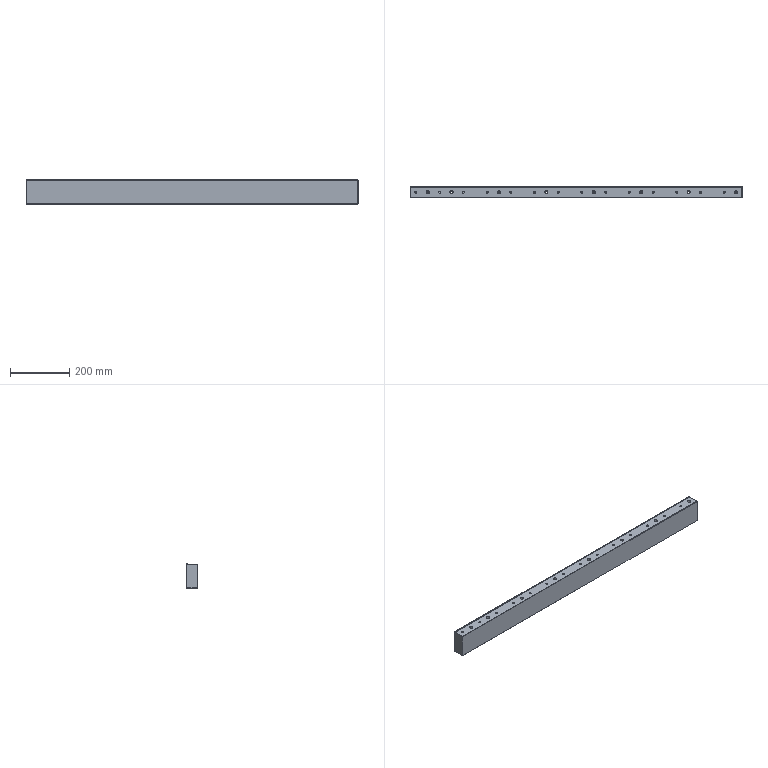Part | STEP file | TJ-DHQM-004-003 | 1 solid | 128 faces | box 1120 x 37.5 x 82.5 mm | volume 3313351 mm3 | cylinder 60 | plane 40 | cone 28 | commonest cylinder face diameters 6.8 x28 6.6 x16 11 x16